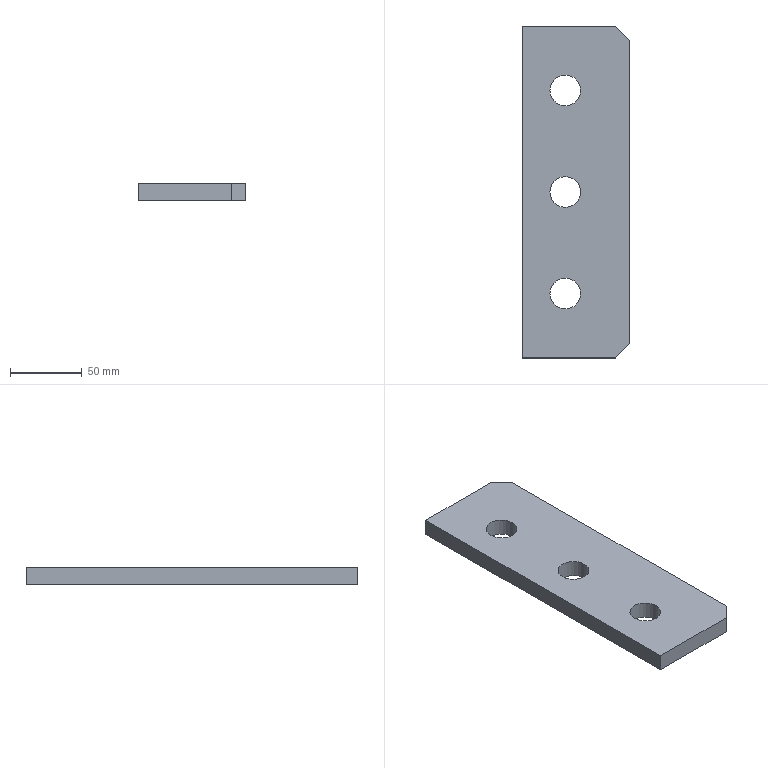Part | STEP file | PN_0021 flange connecting plate 12t_Default<As Machined> | 1 solid | 11 faces | box 75 x 232 x 12 mm | volume 194530 mm3 | plane 8 | cylinder 3 | commonest cylinder face diameters 21.5 x3
STEP:
#1=CARTESIAN_POINT('',(0.,0.,0.));
#2=DIRECTION('',(0.,0.,1.));
#3=DIRECTION('',(1.,0.,0.));
#4=AXIS2_PLACEMENT_3D('',#1,#2,#3);
#5=CARTESIAN_POINT('',(27.5,-116.,0.));
#6=VERTEX_POINT('',#5);
#7=CARTESIAN_POINT('',(27.5,-116.,12.));
#8=VERTEX_POINT('',#7);
#9=CARTESIAN_POINT('',(27.5,-116.,12.));
#10=DIRECTION('',(0.,0.,1.));
#11=VECTOR('',#10,1.);
#12=LINE('',#9,#11);
#13=CARTESIAN_POINT('',(27.5,-116.,12.));
#14=DIRECTION('',(-0.7071,0.7071,0.));
#15=DIRECTION('',(0.,0.,1.));
#16=AXIS2_PLACEMENT_3D('',#13,#14,#15);
#17=PLANE('',#16);
#18=CARTESIAN_POINT('',(0.,0.));
#19=DIRECTION('',(1.,0.));
#20=VECTOR('',#19,1.);
#21=LINE('',#18,#20);
#22=(GEOMETRIC_REPRESENTATION_CONTEXT(2)PARAMETRIC_REPRESENTATION_CONTEXT()REPRESENTATION_CONTEXT('',''));
#23=DEFINITIONAL_REPRESENTATION('',(#21),#22);
#24=PCURVE('',#17,#23);
#25=CARTESIAN_POINT('',(-37.5,-116.,12.));
#26=DIRECTION('',(0.,1.,0.));
#27=DIRECTION('',(0.,0.,1.));
#28=AXIS2_PLACEMENT_3D('',#25,#26,#27);
#29=PLANE('',#28);
#30=CARTESIAN_POINT('',(0.,65.));
#31=DIRECTION('',(1.,0.));
#32=VECTOR('',#31,1.);
#33=LINE('',#30,#32);
#34=(GEOMETRIC_REPRESENTATION_CONTEXT(2)PARAMETRIC_REPRESENTATION_CONTEXT()REPRESENTATION_CONTEXT('',''));
#35=DEFINITIONAL_REPRESENTATION('',(#33),#34);
#36=PCURVE('',#29,#35);
#37=SURFACE_CURVE('',#12,(#24,#36),.PCURVE_S1.);
#38=EDGE_CURVE('',#6,#8,#37,.T.);
#39=ORIENTED_EDGE('',*,*,#38,.F.);
#40=CARTESIAN_POINT('',(37.5,-106.,0.));
#41=VERTEX_POINT('',#40);
#42=CARTESIAN_POINT('',(27.5,-116.,0.));
#43=DIRECTION('',(-0.7071,-0.7071,0.));
#44=VECTOR('',#43,1.);
#45=LINE('',#42,#44);
#46=CARTESIAN_POINT('',(-12.,0.));
#47=DIRECTION('',(0.,-1.));
#48=VECTOR('',#47,1.);
#49=LINE('',#46,#48);
#50=(GEOMETRIC_REPRESENTATION_CONTEXT(2)PARAMETRIC_REPRESENTATION_CONTEXT()REPRESENTATION_CONTEXT('',''));
#51=DEFINITIONAL_REPRESENTATION('',(#49),#50);
#52=PCURVE('',#17,#51);
#53=CARTESIAN_POINT('',(0.,0.,0.));
#54=DIRECTION('',(0.,0.,1.));
#55=DIRECTION('',(1.,0.,0.));
#56=AXIS2_PLACEMENT_3D('',#53,#54,#55);
#57=PLANE('',#56);
#58=CARTESIAN_POINT('',(27.5,-116.));
#59=DIRECTION('',(-0.7071,-0.7071));
#60=VECTOR('',#59,1.);
#61=LINE('',#58,#60);
#62=(GEOMETRIC_REPRESENTATION_CONTEXT(2)PARAMETRIC_REPRESENTATION_CONTEXT()REPRESENTATION_CONTEXT('',''));
#63=DEFINITIONAL_REPRESENTATION('',(#61),#62);
#64=PCURVE('',#57,#63);
#65=SURFACE_CURVE('',#45,(#52,#64),.PCURVE_S1.);
#66=EDGE_CURVE('',#41,#6,#65,.T.);
#67=ORIENTED_EDGE('',*,*,#66,.F.);
#68=CARTESIAN_POINT('',(37.5,-106.,12.));
#69=VERTEX_POINT('',#68);
#70=CARTESIAN_POINT('',(37.5,-106.,12.));
#71=DIRECTION('',(0.,0.,-1.));
#72=VECTOR('',#71,1.);
#73=LINE('',#70,#72);
#74=CARTESIAN_POINT('',(0.,14.142));
#75=DIRECTION('',(-1.,0.));
#76=VECTOR('',#75,1.);
#77=LINE('',#74,#76);
#78=(GEOMETRIC_REPRESENTATION_CONTEXT(2)PARAMETRIC_REPRESENTATION_CONTEXT()REPRESENTATION_CONTEXT('',''));
#79=DEFINITIONAL_REPRESENTATION('',(#77),#78);
#80=PCURVE('',#17,#79);
#81=CARTESIAN_POINT('',(37.5,116.,12.));
#82=DIRECTION('',(-1.,0.,0.));
#83=DIRECTION('',(0.,0.,1.));
#84=AXIS2_PLACEMENT_3D('',#81,#82,#83);
#85=PLANE('',#84);
#86=CARTESIAN_POINT('',(0.,-222.));
#87=DIRECTION('',(-1.,0.));
#88=VECTOR('',#87,1.);
#89=LINE('',#86,#88);
#90=(GEOMETRIC_REPRESENTATION_CONTEXT(2)PARAMETRIC_REPRESENTATION_CONTEXT()REPRESENTATION_CONTEXT('',''));
#91=DEFINITIONAL_REPRESENTATION('',(#89),#90);
#92=PCURVE('',#85,#91);
#93=SURFACE_CURVE('',#73,(#80,#92),.PCURVE_S1.);
#94=EDGE_CURVE('',#69,#41,#93,.T.);
#95=ORIENTED_EDGE('',*,*,#94,.F.);
#96=CARTESIAN_POINT('',(71.75,-71.75,12.));
#97=DIRECTION('',(0.7071,0.7071,0.));
#98=VECTOR('',#97,1.);
#99=LINE('',#96,#98);
#100=CARTESIAN_POINT('',(0.,62.579));
#101=DIRECTION('',(0.,1.));
#102=VECTOR('',#101,1.);
#103=LINE('',#100,#102);
#104=(GEOMETRIC_REPRESENTATION_CONTEXT(2)PARAMETRIC_REPRESENTATION_CONTEXT()REPRESENTATION_CONTEXT('',''));
#105=DEFINITIONAL_REPRESENTATION('',(#103),#104);
#106=PCURVE('',#17,#105);
#107=CARTESIAN_POINT('',(0.,0.,12.));
#108=DIRECTION('',(0.,0.,1.));
#109=DIRECTION('',(1.,0.,0.));
#110=AXIS2_PLACEMENT_3D('',#107,#108,#109);
#111=PLANE('',#110);
#112=CARTESIAN_POINT('',(71.75,-71.75));
#113=DIRECTION('',(0.7071,0.7071));
#114=VECTOR('',#113,1.);
#115=LINE('',#112,#114);
#116=(GEOMETRIC_REPRESENTATION_CONTEXT(2)PARAMETRIC_REPRESENTATION_CONTEXT()REPRESENTATION_CONTEXT('',''));
#117=DEFINITIONAL_REPRESENTATION('',(#115),#116);
#118=PCURVE('',#111,#117);
#119=SURFACE_CURVE('',#99,(#106,#118),.PCURVE_S1.);
#120=EDGE_CURVE('',#8,#69,#119,.T.);
#121=ORIENTED_EDGE('',*,*,#120,.F.);
#122=EDGE_LOOP('',(#39,#67,#95,#121));
#123=FACE_BOUND('',#122,.T.);
#124=ADVANCED_FACE('',(#123),#17,.F.);
#125=CARTESIAN_POINT('',(27.5,116.,12.));
#126=VERTEX_POINT('',#125);
#127=CARTESIAN_POINT('',(27.5,116.,0.));
#128=VERTEX_POINT('',#127);
#129=CARTESIAN_POINT('',(27.5,116.,12.));
#130=DIRECTION('',(0.,0.,-1.));
#131=VECTOR('',#130,1.);
#132=LINE('',#129,#131);
#133=CARTESIAN_POINT('',(27.5,116.,12.));
#134=DIRECTION('',(-0.7071,-0.7071,0.));
#135=DIRECTION('',(0.,0.,-1.));
#136=AXIS2_PLACEMENT_3D('',#133,#134,#135);
#137=PLANE('',#136);
#138=CARTESIAN_POINT('',(0.,0.));
#139=DIRECTION('',(1.,0.));
#140=VECTOR('',#139,1.);
#141=LINE('',#138,#140);
#142=(GEOMETRIC_REPRESENTATION_CONTEXT(2)PARAMETRIC_REPRESENTATION_CONTEXT()REPRESENTATION_CONTEXT('',''));
#143=DEFINITIONAL_REPRESENTATION('',(#141),#142);
#144=PCURVE('',#137,#143);
#145=CARTESIAN_POINT('',(-37.5,116.,12.));
#146=DIRECTION('',(0.,-1.,0.));
#147=DIRECTION('',(0.,0.,-1.));
#148=AXIS2_PLACEMENT_3D('',#145,#146,#147);
#149=PLANE('',#148);
#150=CARTESIAN_POINT('',(0.,65.));
#151=DIRECTION('',(1.,0.));
#152=VECTOR('',#151,1.);
#153=LINE('',#150,#152);
#154=(GEOMETRIC_REPRESENTATION_CONTEXT(2)PARAMETRIC_REPRESENTATION_CONTEXT()REPRESENTATION_CONTEXT('',''));
#155=DEFINITIONAL_REPRESENTATION('',(#153),#154);
#156=PCURVE('',#149,#155);
#157=SURFACE_CURVE('',#132,(#144,#156),.PCURVE_S1.);
#158=EDGE_CURVE('',#126,#128,#157,.T.);
#159=ORIENTED_EDGE('',*,*,#158,.F.);
#160=CARTESIAN_POINT('',(37.5,106.,12.));
#161=VERTEX_POINT('',#160);
#162=CARTESIAN_POINT('',(71.75,71.75,12.));
#163=DIRECTION('',(-0.7071,0.7071,0.));
#164=VECTOR('',#163,1.);
#165=LINE('',#162,#164);
#166=CARTESIAN_POINT('',(0.,62.579));
#167=DIRECTION('',(0.,-1.));
#168=VECTOR('',#167,1.);
#169=LINE('',#166,#168);
#170=(GEOMETRIC_REPRESENTATION_CONTEXT(2)PARAMETRIC_REPRESENTATION_CONTEXT()REPRESENTATION_CONTEXT('',''));
#171=DEFINITIONAL_REPRESENTATION('',(#169),#170);
#172=PCURVE('',#137,#171);
#173=CARTESIAN_POINT('',(71.75,71.75));
#174=DIRECTION('',(-0.7071,0.7071));
#175=VECTOR('',#174,1.);
#176=LINE('',#173,#175);
#177=(GEOMETRIC_REPRESENTATION_CONTEXT(2)PARAMETRIC_REPRESENTATION_CONTEXT()REPRESENTATION_CONTEXT('',''));
#178=DEFINITIONAL_REPRESENTATION('',(#176),#177);
#179=PCURVE('',#111,#178);
#180=SURFACE_CURVE('',#165,(#172,#179),.PCURVE_S1.);
#181=EDGE_CURVE('',#161,#126,#180,.T.);
#182=ORIENTED_EDGE('',*,*,#181,.F.);
#183=CARTESIAN_POINT('',(37.5,106.,0.));
#184=VERTEX_POINT('',#183);
#185=CARTESIAN_POINT('',(37.5,106.,12.));
#186=DIRECTION('',(0.,0.,1.));
#187=VECTOR('',#186,1.);
#188=LINE('',#185,#187);
#189=CARTESIAN_POINT('',(0.,14.142));
#190=DIRECTION('',(-1.,0.));
#191=VECTOR('',#190,1.);
#192=LINE('',#189,#191);
#193=(GEOMETRIC_REPRESENTATION_CONTEXT(2)PARAMETRIC_REPRESENTATION_CONTEXT()REPRESENTATION_CONTEXT('',''));
#194=DEFINITIONAL_REPRESENTATION('',(#192),#193);
#195=PCURVE('',#137,#194);
#196=CARTESIAN_POINT('',(0.,-10.));
#197=DIRECTION('',(1.,0.));
#198=VECTOR('',#197,1.);
#199=LINE('',#196,#198);
#200=(GEOMETRIC_REPRESENTATION_CONTEXT(2)PARAMETRIC_REPRESENTATION_CONTEXT()REPRESENTATION_CONTEXT('',''));
#201=DEFINITIONAL_REPRESENTATION('',(#199),#200);
#202=PCURVE('',#85,#201);
#203=SURFACE_CURVE('',#188,(#195,#202),.PCURVE_S1.);
#204=EDGE_CURVE('',#184,#161,#203,.T.);
#205=ORIENTED_EDGE('',*,*,#204,.F.);
#206=CARTESIAN_POINT('',(27.5,116.,0.));
#207=DIRECTION('',(0.7071,-0.7071,0.));
#208=VECTOR('',#207,1.);
#209=LINE('',#206,#208);
#210=CARTESIAN_POINT('',(12.,0.));
#211=DIRECTION('',(0.,1.));
#212=VECTOR('',#211,1.);
#213=LINE('',#210,#212);
#214=(GEOMETRIC_REPRESENTATION_CONTEXT(2)PARAMETRIC_REPRESENTATION_CONTEXT()REPRESENTATION_CONTEXT('',''));
#215=DEFINITIONAL_REPRESENTATION('',(#213),#214);
#216=PCURVE('',#137,#215);
#217=CARTESIAN_POINT('',(27.5,116.));
#218=DIRECTION('',(0.7071,-0.7071));
#219=VECTOR('',#218,1.);
#220=LINE('',#217,#219);
#221=(GEOMETRIC_REPRESENTATION_CONTEXT(2)PARAMETRIC_REPRESENTATION_CONTEXT()REPRESENTATION_CONTEXT('',''));
#222=DEFINITIONAL_REPRESENTATION('',(#220),#221);
#223=PCURVE('',#57,#222);
#224=SURFACE_CURVE('',#209,(#216,#223),.PCURVE_S1.);
#225=EDGE_CURVE('',#128,#184,#224,.T.);
#226=ORIENTED_EDGE('',*,*,#225,.F.);
#227=EDGE_LOOP('',(#159,#182,#205,#226));
#228=FACE_BOUND('',#227,.T.);
#229=ADVANCED_FACE('',(#228),#137,.F.);
#230=CARTESIAN_POINT('',(37.5,116.,12.));
#231=DIRECTION('',(0.,1.,0.));
#232=VECTOR('',#231,1.);
#233=LINE('',#230,#232);
#234=CARTESIAN_POINT('',(0.,0.));
#235=DIRECTION('',(0.,1.));
#236=VECTOR('',#235,1.);
#237=LINE('',#234,#236);
#238=(GEOMETRIC_REPRESENTATION_CONTEXT(2)PARAMETRIC_REPRESENTATION_CONTEXT()REPRESENTATION_CONTEXT('',''));
#239=DEFINITIONAL_REPRESENTATION('',(#237),#238);
#240=PCURVE('',#85,#239);
#241=CARTESIAN_POINT('',(37.5,116.));
#242=DIRECTION('',(0.,1.));
#243=VECTOR('',#242,1.);
#244=LINE('',#241,#243);
#245=(GEOMETRIC_REPRESENTATION_CONTEXT(2)PARAMETRIC_REPRESENTATION_CONTEXT()REPRESENTATION_CONTEXT('',''));
#246=DEFINITIONAL_REPRESENTATION('',(#244),#245);
#247=PCURVE('',#111,#246);
#248=SURFACE_CURVE('',#233,(#240,#247),.PCURVE_S1.);
#249=EDGE_CURVE('',#69,#161,#248,.T.);
#250=ORIENTED_EDGE('',*,*,#249,.F.);
#251=ORIENTED_EDGE('',*,*,#94,.T.);
#252=CARTESIAN_POINT('',(37.5,116.,0.));
#253=DIRECTION('',(0.,1.,0.));
#254=VECTOR('',#253,1.);
#255=LINE('',#252,#254);
#256=CARTESIAN_POINT('',(-12.,0.));
#257=DIRECTION('',(0.,1.));
#258=VECTOR('',#257,1.);
#259=LINE('',#256,#258);
#260=(GEOMETRIC_REPRESENTATION_CONTEXT(2)PARAMETRIC_REPRESENTATION_CONTEXT()REPRESENTATION_CONTEXT('',''));
#261=DEFINITIONAL_REPRESENTATION('',(#259),#260);
#262=PCURVE('',#85,#261);
#263=CARTESIAN_POINT('',(37.5,116.));
#264=DIRECTION('',(0.,1.));
#265=VECTOR('',#264,1.);
#266=LINE('',#263,#265);
#267=(GEOMETRIC_REPRESENTATION_CONTEXT(2)PARAMETRIC_REPRESENTATION_CONTEXT()REPRESENTATION_CONTEXT('',''));
#268=DEFINITIONAL_REPRESENTATION('',(#266),#267);
#269=PCURVE('',#57,#268);
#270=SURFACE_CURVE('',#255,(#262,#269),.PCURVE_S1.);
#271=EDGE_CURVE('',#41,#184,#270,.T.);
#272=ORIENTED_EDGE('',*,*,#271,.T.);
#273=ORIENTED_EDGE('',*,*,#204,.T.);
#274=EDGE_LOOP('',(#250,#251,#272,#273));
#275=FACE_BOUND('',#274,.T.);
#276=ADVANCED_FACE('',(#275),#85,.F.);
#277=CARTESIAN_POINT('',(-37.5,116.,12.));
#278=VERTEX_POINT('',#277);
#279=CARTESIAN_POINT('',(-37.5,116.,12.));
#280=DIRECTION('',(-1.,0.,0.));
#281=VECTOR('',#280,1.);
#282=LINE('',#279,#281);
#283=CARTESIAN_POINT('',(0.,0.));
#284=DIRECTION('',(0.,-1.));
#285=VECTOR('',#284,1.);
#286=LINE('',#283,#285);
#287=(GEOMETRIC_REPRESENTATION_CONTEXT(2)PARAMETRIC_REPRESENTATION_CONTEXT()REPRESENTATION_CONTEXT('',''));
#288=DEFINITIONAL_REPRESENTATION('',(#286),#287);
#289=PCURVE('',#149,#288);
#290=CARTESIAN_POINT('',(-37.5,116.));
#291=DIRECTION('',(-1.,0.));
#292=VECTOR('',#291,1.);
#293=LINE('',#290,#292);
#294=(GEOMETRIC_REPRESENTATION_CONTEXT(2)PARAMETRIC_REPRESENTATION_CONTEXT()REPRESENTATION_CONTEXT('',''));
#295=DEFINITIONAL_REPRESENTATION('',(#293),#294);
#296=PCURVE('',#111,#295);
#297=SURFACE_CURVE('',#282,(#289,#296),.PCURVE_S1.);
#298=EDGE_CURVE('',#126,#278,#297,.T.);
#299=ORIENTED_EDGE('',*,*,#298,.F.);
#300=ORIENTED_EDGE('',*,*,#158,.T.);
#301=CARTESIAN_POINT('',(-37.5,116.,0.));
#302=VERTEX_POINT('',#301);
#303=CARTESIAN_POINT('',(-37.5,116.,0.));
#304=DIRECTION('',(-1.,0.,0.));
#305=VECTOR('',#304,1.);
#306=LINE('',#303,#305);
#307=CARTESIAN_POINT('',(12.,0.));
#308=DIRECTION('',(0.,-1.));
#309=VECTOR('',#308,1.);
#310=LINE('',#307,#309);
#311=(GEOMETRIC_REPRESENTATION_CONTEXT(2)PARAMETRIC_REPRESENTATION_CONTEXT()REPRESENTATION_CONTEXT('',''));
#312=DEFINITIONAL_REPRESENTATION('',(#310),#311);
#313=PCURVE('',#149,#312);
#314=CARTESIAN_POINT('',(-37.5,116.));
#315=DIRECTION('',(-1.,0.));
#316=VECTOR('',#315,1.);
#317=LINE('',#314,#316);
#318=(GEOMETRIC_REPRESENTATION_CONTEXT(2)PARAMETRIC_REPRESENTATION_CONTEXT()REPRESENTATION_CONTEXT('',''));
#319=DEFINITIONAL_REPRESENTATION('',(#317),#318);
#320=PCURVE('',#57,#319);
#321=SURFACE_CURVE('',#306,(#313,#320),.PCURVE_S1.);
#322=EDGE_CURVE('',#128,#302,#321,.T.);
#323=ORIENTED_EDGE('',*,*,#322,.T.);
#324=CARTESIAN_POINT('',(-37.5,116.,12.));
#325=DIRECTION('',(0.,0.,-1.));
#326=VECTOR('',#325,1.);
#327=LINE('',#324,#326);
#328=CARTESIAN_POINT('',(0.,0.));
#329=DIRECTION('',(1.,0.));
#330=VECTOR('',#329,1.);
#331=LINE('',#328,#330);
#332=(GEOMETRIC_REPRESENTATION_CONTEXT(2)PARAMETRIC_REPRESENTATION_CONTEXT()REPRESENTATION_CONTEXT('',''));
#333=DEFINITIONAL_REPRESENTATION('',(#331),#332);
#334=PCURVE('',#149,#333);
#335=CARTESIAN_POINT('',(-37.5,116.,12.));
#336=DIRECTION('',(1.,0.,0.));
#337=DIRECTION('',(0.,0.,-1.));
#338=AXIS2_PLACEMENT_3D('',#335,#336,#337);
#339=PLANE('',#338);
#340=CARTESIAN_POINT('',(0.,0.));
#341=DIRECTION('',(1.,0.));
#342=VECTOR('',#341,1.);
#343=LINE('',#340,#342);
#344=(GEOMETRIC_REPRESENTATION_CONTEXT(2)PARAMETRIC_REPRESENTATION_CONTEXT()REPRESENTATION_CONTEXT('',''));
#345=DEFINITIONAL_REPRESENTATION('',(#343),#344);
#346=PCURVE('',#339,#345);
#347=SURFACE_CURVE('',#327,(#334,#346),.PCURVE_S1.);
#348=EDGE_CURVE('',#278,#302,#347,.T.);
#349=ORIENTED_EDGE('',*,*,#348,.F.);
#350=EDGE_LOOP('',(#299,#300,#323,#349));
#351=FACE_BOUND('',#350,.T.);
#352=ADVANCED_FACE('',(#351),#149,.F.);
#353=CARTESIAN_POINT('',(-37.5,-116.,0.));
#354=VERTEX_POINT('',#353);
#355=CARTESIAN_POINT('',(-37.5,116.,0.));
#356=DIRECTION('',(0.,-1.,0.));
#357=VECTOR('',#356,1.);
#358=LINE('',#355,#357);
#359=CARTESIAN_POINT('',(12.,0.));
#360=DIRECTION('',(0.,-1.));
#361=VECTOR('',#360,1.);
#362=LINE('',#359,#361);
#363=(GEOMETRIC_REPRESENTATION_CONTEXT(2)PARAMETRIC_REPRESENTATION_CONTEXT()REPRESENTATION_CONTEXT('',''));
#364=DEFINITIONAL_REPRESENTATION('',(#362),#363);
#365=PCURVE('',#339,#364);
#366=CARTESIAN_POINT('',(-37.5,116.));
#367=DIRECTION('',(0.,-1.));
#368=VECTOR('',#367,1.);
#369=LINE('',#366,#368);
#370=(GEOMETRIC_REPRESENTATION_CONTEXT(2)PARAMETRIC_REPRESENTATION_CONTEXT()REPRESENTATION_CONTEXT('',''));
#371=DEFINITIONAL_REPRESENTATION('',(#369),#370);
#372=PCURVE('',#57,#371);
#373=SURFACE_CURVE('',#358,(#365,#372),.PCURVE_S1.);
#374=EDGE_CURVE('',#302,#354,#373,.T.);
#375=ORIENTED_EDGE('',*,*,#374,.T.);
#376=CARTESIAN_POINT('',(-37.5,-116.,12.));
#377=VERTEX_POINT('',#376);
#378=CARTESIAN_POINT('',(-37.5,-116.,12.));
#379=DIRECTION('',(0.,0.,-1.));
#380=VECTOR('',#379,1.);
#381=LINE('',#378,#380);
#382=CARTESIAN_POINT('',(0.,-232.));
#383=DIRECTION('',(1.,0.));
#384=VECTOR('',#383,1.);
#385=LINE('',#382,#384);
#386=(GEOMETRIC_REPRESENTATION_CONTEXT(2)PARAMETRIC_REPRESENTATION_CONTEXT()REPRESENTATION_CONTEXT('',''));
#387=DEFINITIONAL_REPRESENTATION('',(#385),#386);
#388=PCURVE('',#339,#387);
#389=CARTESIAN_POINT('',(0.,0.));
#390=DIRECTION('',(-1.,0.));
#391=VECTOR('',#390,1.);
#392=LINE('',#389,#391);
#393=(GEOMETRIC_REPRESENTATION_CONTEXT(2)PARAMETRIC_REPRESENTATION_CONTEXT()REPRESENTATION_CONTEXT('',''));
#394=DEFINITIONAL_REPRESENTATION('',(#392),#393);
#395=PCURVE('',#29,#394);
#396=SURFACE_CURVE('',#381,(#388,#395),.PCURVE_S1.);
#397=EDGE_CURVE('',#377,#354,#396,.T.);
#398=ORIENTED_EDGE('',*,*,#397,.F.);
#399=CARTESIAN_POINT('',(-37.5,116.,12.));
#400=DIRECTION('',(0.,-1.,0.));
#401=VECTOR('',#400,1.);
#402=LINE('',#399,#401);
#403=CARTESIAN_POINT('',(0.,0.));
#404=DIRECTION('',(0.,-1.));
#405=VECTOR('',#404,1.);
#406=LINE('',#403,#405);
#407=(GEOMETRIC_REPRESENTATION_CONTEXT(2)PARAMETRIC_REPRESENTATION_CONTEXT()REPRESENTATION_CONTEXT('',''));
#408=DEFINITIONAL_REPRESENTATION('',(#406),#407);
#409=PCURVE('',#339,#408);
#410=CARTESIAN_POINT('',(-37.5,116.));
#411=DIRECTION('',(0.,-1.));
#412=VECTOR('',#411,1.);
#413=LINE('',#410,#412);
#414=(GEOMETRIC_REPRESENTATION_CONTEXT(2)PARAMETRIC_REPRESENTATION_CONTEXT()REPRESENTATION_CONTEXT('',''));
#415=DEFINITIONAL_REPRESENTATION('',(#413),#414);
#416=PCURVE('',#111,#415);
#417=SURFACE_CURVE('',#402,(#409,#416),.PCURVE_S1.);
#418=EDGE_CURVE('',#278,#377,#417,.T.);
#419=ORIENTED_EDGE('',*,*,#418,.F.);
#420=ORIENTED_EDGE('',*,*,#348,.T.);
#421=EDGE_LOOP('',(#375,#398,#419,#420));
#422=FACE_BOUND('',#421,.T.);
#423=ADVANCED_FACE('',(#422),#339,.F.);
#424=CARTESIAN_POINT('',(-37.5,-116.,0.));
#425=DIRECTION('',(1.,0.,0.));
#426=VECTOR('',#425,1.);
#427=LINE('',#424,#426);
#428=CARTESIAN_POINT('',(-12.,0.));
#429=DIRECTION('',(0.,1.));
#430=VECTOR('',#429,1.);
#431=LINE('',#428,#430);
#432=(GEOMETRIC_REPRESENTATION_CONTEXT(2)PARAMETRIC_REPRESENTATION_CONTEXT()REPRESENTATION_CONTEXT('',''));
#433=DEFINITIONAL_REPRESENTATION('',(#431),#432);
#434=PCURVE('',#29,#433);
#435=CARTESIAN_POINT('',(-37.5,-116.));
#436=DIRECTION('',(1.,0.));
#437=VECTOR('',#436,1.);
#438=LINE('',#435,#437);
#439=(GEOMETRIC_REPRESENTATION_CONTEXT(2)PARAMETRIC_REPRESENTATION_CONTEXT()REPRESENTATION_CONTEXT('',''));
#440=DEFINITIONAL_REPRESENTATION('',(#438),#439);
#441=PCURVE('',#57,#440);
#442=SURFACE_CURVE('',#427,(#434,#441),.PCURVE_S1.);
#443=EDGE_CURVE('',#354,#6,#442,.T.);
#444=ORIENTED_EDGE('',*,*,#443,.T.);
#445=ORIENTED_EDGE('',*,*,#38,.T.);
#446=CARTESIAN_POINT('',(-37.5,-116.,12.));
#447=DIRECTION('',(1.,0.,0.));
#448=VECTOR('',#447,1.);
#449=LINE('',#446,#448);
#450=CARTESIAN_POINT('',(0.,0.));
#451=DIRECTION('',(0.,1.));
#452=VECTOR('',#451,1.);
#453=LINE('',#450,#452);
#454=(GEOMETRIC_REPRESENTATION_CONTEXT(2)PARAMETRIC_REPRESENTATION_CONTEXT()REPRESENTATION_CONTEXT('',''));
#455=DEFINITIONAL_REPRESENTATION('',(#453),#454);
#456=PCURVE('',#29,#455);
#457=CARTESIAN_POINT('',(-37.5,-116.));
#458=DIRECTION('',(1.,0.));
#459=VECTOR('',#458,1.);
#460=LINE('',#457,#459);
#461=(GEOMETRIC_REPRESENTATION_CONTEXT(2)PARAMETRIC_REPRESENTATION_CONTEXT()REPRESENTATION_CONTEXT('',''));
#462=DEFINITIONAL_REPRESENTATION('',(#460),#461);
#463=PCURVE('',#111,#462);
#464=SURFACE_CURVE('',#449,(#456,#463),.PCURVE_S1.);
#465=EDGE_CURVE('',#377,#8,#464,.T.);
#466=ORIENTED_EDGE('',*,*,#465,.F.);
#467=ORIENTED_EDGE('',*,*,#397,.T.);
#468=EDGE_LOOP('',(#444,#445,#466,#467));
#469=FACE_BOUND('',#468,.T.);
#470=ADVANCED_FACE('',(#469),#29,.F.);
#471=CARTESIAN_POINT('',(3.25,71.,12.));
#472=VERTEX_POINT('',#471);
#473=CARTESIAN_POINT('',(-7.5,71.,12.));
#474=DIRECTION('',(0.,0.,1.));
#475=DIRECTION('',(1.,0.,0.));
#476=AXIS2_PLACEMENT_3D('',#473,#474,#475);
#477=CIRCLE('',#476,10.75);
#478=CARTESIAN_POINT('',(-7.5,71.));
#479=DIRECTION('',(1.,0.));
#480=AXIS2_PLACEMENT_2D('',#478,#479);
#481=CIRCLE('',#480,10.75);
#482=(GEOMETRIC_REPRESENTATION_CONTEXT(2)PARAMETRIC_REPRESENTATION_CONTEXT()REPRESENTATION_CONTEXT('',''));
#483=DEFINITIONAL_REPRESENTATION('',(#481),#482);
#484=PCURVE('',#111,#483);
#485=CARTESIAN_POINT('',(-7.5,71.,12.));
#486=DIRECTION('',(0.,0.,1.));
#487=DIRECTION('',(1.,0.,0.));
#488=AXIS2_PLACEMENT_3D('',#485,#486,#487);
#489=CYLINDRICAL_SURFACE('',#488,10.75);
#490=CARTESIAN_POINT('',(0.,0.));
#491=DIRECTION('',(1.,0.));
#492=VECTOR('',#491,1.);
#493=LINE('',#490,#492);
#494=(GEOMETRIC_REPRESENTATION_CONTEXT(2)PARAMETRIC_REPRESENTATION_CONTEXT()REPRESENTATION_CONTEXT('',''));
#495=DEFINITIONAL_REPRESENTATION('',(#493),#494);
#496=PCURVE('',#489,#495);
#497=SURFACE_CURVE('',#477,(#484,#496),.PCURVE_S1.);
#498=EDGE_CURVE('',#472,#472,#497,.T.);
#499=ORIENTED_EDGE('',*,*,#498,.F.);
#500=EDGE_LOOP('',(#499));
#501=FACE_BOUND('',#500,.T.);
#502=CARTESIAN_POINT('',(3.25,0.,12.));
#503=VERTEX_POINT('',#502);
#504=CARTESIAN_POINT('',(-7.5,0.,12.));
#505=DIRECTION('',(0.,0.,1.));
#506=DIRECTION('',(1.,0.,0.));
#507=AXIS2_PLACEMENT_3D('',#504,#505,#506);
#508=CIRCLE('',#507,10.75);
#509=CARTESIAN_POINT('',(-7.5,0.));
#510=DIRECTION('',(1.,0.));
#511=AXIS2_PLACEMENT_2D('',#509,#510);
#512=CIRCLE('',#511,10.75);
#513=(GEOMETRIC_REPRESENTATION_CONTEXT(2)PARAMETRIC_REPRESENTATION_CONTEXT()REPRESENTATION_CONTEXT('',''));
#514=DEFINITIONAL_REPRESENTATION('',(#512),#513);
#515=PCURVE('',#111,#514);
#516=CARTESIAN_POINT('',(-7.5,0.,12.));
#517=DIRECTION('',(0.,0.,1.));
#518=DIRECTION('',(1.,0.,0.));
#519=AXIS2_PLACEMENT_3D('',#516,#517,#518);
#520=CYLINDRICAL_SURFACE('',#519,10.75);
#521=CARTESIAN_POINT('',(0.,0.));
#522=DIRECTION('',(1.,0.));
#523=VECTOR('',#522,1.);
#524=LINE('',#521,#523);
#525=(GEOMETRIC_REPRESENTATION_CONTEXT(2)PARAMETRIC_REPRESENTATION_CONTEXT()REPRESENTATION_CONTEXT('',''));
#526=DEFINITIONAL_REPRESENTATION('',(#524),#525);
#527=PCURVE('',#520,#526);
#528=SURFACE_CURVE('',#508,(#515,#527),.PCURVE_S1.);
#529=EDGE_CURVE('',#503,#503,#528,.T.);
#530=ORIENTED_EDGE('',*,*,#529,.F.);
#531=EDGE_LOOP('',(#530));
#532=FACE_BOUND('',#531,.T.);
#533=CARTESIAN_POINT('',(3.25,-71.,12.));
#534=VERTEX_POINT('',#533);
#535=CARTESIAN_POINT('',(-7.5,-71.,12.));
#536=DIRECTION('',(0.,0.,1.));
#537=DIRECTION('',(1.,0.,0.));
#538=AXIS2_PLACEMENT_3D('',#535,#536,#537);
#539=CIRCLE('',#538,10.75);
#540=CARTESIAN_POINT('',(-7.5,-71.));
#541=DIRECTION('',(1.,0.));
#542=AXIS2_PLACEMENT_2D('',#540,#541);
#543=CIRCLE('',#542,10.75);
#544=(GEOMETRIC_REPRESENTATION_CONTEXT(2)PARAMETRIC_REPRESENTATION_CONTEXT()REPRESENTATION_CONTEXT('',''));
#545=DEFINITIONAL_REPRESENTATION('',(#543),#544);
#546=PCURVE('',#111,#545);
#547=CARTESIAN_POINT('',(-7.5,-71.,12.));
#548=DIRECTION('',(0.,0.,1.));
#549=DIRECTION('',(1.,0.,0.));
#550=AXIS2_PLACEMENT_3D('',#547,#548,#549);
#551=CYLINDRICAL_SURFACE('',#550,10.75);
#552=CARTESIAN_POINT('',(0.,0.));
#553=DIRECTION('',(1.,0.));
#554=VECTOR('',#553,1.);
#555=LINE('',#552,#554);
#556=(GEOMETRIC_REPRESENTATION_CONTEXT(2)PARAMETRIC_REPRESENTATION_CONTEXT()REPRESENTATION_CONTEXT('',''));
#557=DEFINITIONAL_REPRESENTATION('',(#555),#556);
#558=PCURVE('',#551,#557);
#559=SURFACE_CURVE('',#539,(#546,#558),.PCURVE_S1.);
#560=EDGE_CURVE('',#534,#534,#559,.T.);
#561=ORIENTED_EDGE('',*,*,#560,.F.);
#562=EDGE_LOOP('',(#561));
#563=FACE_BOUND('',#562,.T.);
#564=ORIENTED_EDGE('',*,*,#465,.T.);
#565=ORIENTED_EDGE('',*,*,#120,.T.);
#566=ORIENTED_EDGE('',*,*,#249,.T.);
#567=ORIENTED_EDGE('',*,*,#181,.T.);
#568=ORIENTED_EDGE('',*,*,#298,.T.);
#569=ORIENTED_EDGE('',*,*,#418,.T.);
#570=EDGE_LOOP('',(#564,#565,#566,#567,#568,#569));
#571=FACE_BOUND('',#570,.T.);
#572=ADVANCED_FACE('',(#501,#532,#563,#571),#111,.T.);
#573=CARTESIAN_POINT('',(3.25,71.,0.));
#574=VERTEX_POINT('',#573);
#575=CARTESIAN_POINT('',(-7.5,71.,0.));
#576=DIRECTION('',(0.,0.,1.));
#577=DIRECTION('',(1.,0.,0.));
#578=AXIS2_PLACEMENT_3D('',#575,#576,#577);
#579=CIRCLE('',#578,10.75);
#580=CARTESIAN_POINT('',(-7.5,71.));
#581=DIRECTION('',(1.,0.));
#582=AXIS2_PLACEMENT_2D('',#580,#581);
#583=CIRCLE('',#582,10.75);
#584=(GEOMETRIC_REPRESENTATION_CONTEXT(2)PARAMETRIC_REPRESENTATION_CONTEXT()REPRESENTATION_CONTEXT('',''));
#585=DEFINITIONAL_REPRESENTATION('',(#583),#584);
#586=PCURVE('',#57,#585);
#587=CARTESIAN_POINT('',(0.,-12.));
#588=DIRECTION('',(1.,0.));
#589=VECTOR('',#588,1.);
#590=LINE('',#587,#589);
#591=(GEOMETRIC_REPRESENTATION_CONTEXT(2)PARAMETRIC_REPRESENTATION_CONTEXT()REPRESENTATION_CONTEXT('',''));
#592=DEFINITIONAL_REPRESENTATION('',(#590),#591);
#593=PCURVE('',#489,#592);
#594=SURFACE_CURVE('',#579,(#586,#593),.PCURVE_S1.);
#595=EDGE_CURVE('',#574,#574,#594,.T.);
#596=ORIENTED_EDGE('',*,*,#595,.T.);
#597=EDGE_LOOP('',(#596));
#598=FACE_BOUND('',#597,.T.);
#599=CARTESIAN_POINT('',(3.25,0.,0.));
#600=VERTEX_POINT('',#599);
#601=CARTESIAN_POINT('',(-7.5,0.,0.));
#602=DIRECTION('',(0.,0.,1.));
#603=DIRECTION('',(1.,0.,0.));
#604=AXIS2_PLACEMENT_3D('',#601,#602,#603);
#605=CIRCLE('',#604,10.75);
#606=CARTESIAN_POINT('',(-7.5,0.));
#607=DIRECTION('',(1.,0.));
#608=AXIS2_PLACEMENT_2D('',#606,#607);
#609=CIRCLE('',#608,10.75);
#610=(GEOMETRIC_REPRESENTATION_CONTEXT(2)PARAMETRIC_REPRESENTATION_CONTEXT()REPRESENTATION_CONTEXT('',''));
#611=DEFINITIONAL_REPRESENTATION('',(#609),#610);
#612=PCURVE('',#57,#611);
#613=CARTESIAN_POINT('',(0.,-12.));
#614=DIRECTION('',(1.,0.));
#615=VECTOR('',#614,1.);
#616=LINE('',#613,#615);
#617=(GEOMETRIC_REPRESENTATION_CONTEXT(2)PARAMETRIC_REPRESENTATION_CONTEXT()REPRESENTATION_CONTEXT('',''));
#618=DEFINITIONAL_REPRESENTATION('',(#616),#617);
#619=PCURVE('',#520,#618);
#620=SURFACE_CURVE('',#605,(#612,#619),.PCURVE_S1.);
#621=EDGE_CURVE('',#600,#600,#620,.T.);
#622=ORIENTED_EDGE('',*,*,#621,.T.);
#623=EDGE_LOOP('',(#622));
#624=FACE_BOUND('',#623,.T.);
#625=CARTESIAN_POINT('',(3.25,-71.,0.));
#626=VERTEX_POINT('',#625);
#627=CARTESIAN_POINT('',(-7.5,-71.,0.));
#628=DIRECTION('',(0.,0.,1.));
#629=DIRECTION('',(1.,0.,0.));
#630=AXIS2_PLACEMENT_3D('',#627,#628,#629);
#631=CIRCLE('',#630,10.75);
#632=CARTESIAN_POINT('',(-7.5,-71.));
#633=DIRECTION('',(1.,0.));
#634=AXIS2_PLACEMENT_2D('',#632,#633);
#635=CIRCLE('',#634,10.75);
#636=(GEOMETRIC_REPRESENTATION_CONTEXT(2)PARAMETRIC_REPRESENTATION_CONTEXT()REPRESENTATION_CONTEXT('',''));
#637=DEFINITIONAL_REPRESENTATION('',(#635),#636);
#638=PCURVE('',#57,#637);
#639=CARTESIAN_POINT('',(0.,-12.));
#640=DIRECTION('',(1.,0.));
#641=VECTOR('',#640,1.);
#642=LINE('',#639,#641);
#643=(GEOMETRIC_REPRESENTATION_CONTEXT(2)PARAMETRIC_REPRESENTATION_CONTEXT()REPRESENTATION_CONTEXT('',''));
#644=DEFINITIONAL_REPRESENTATION('',(#642),#643);
#645=PCURVE('',#551,#644);
#646=SURFACE_CURVE('',#631,(#638,#645),.PCURVE_S1.);
#647=EDGE_CURVE('',#626,#626,#646,.T.);
#648=ORIENTED_EDGE('',*,*,#647,.T.);
#649=EDGE_LOOP('',(#648));
#650=FACE_BOUND('',#649,.T.);
#651=ORIENTED_EDGE('',*,*,#271,.F.);
#652=ORIENTED_EDGE('',*,*,#66,.T.);
#653=ORIENTED_EDGE('',*,*,#443,.F.);
#654=ORIENTED_EDGE('',*,*,#374,.F.);
#655=ORIENTED_EDGE('',*,*,#322,.F.);
#656=ORIENTED_EDGE('',*,*,#225,.T.);
#657=EDGE_LOOP('',(#651,#652,#653,#654,#655,#656));
#658=FACE_BOUND('',#657,.T.);
#659=ADVANCED_FACE('',(#598,#624,#650,#658),#57,.F.);
#660=ORIENTED_EDGE('',*,*,#560,.F.);
#661=CARTESIAN_POINT('',(3.25,-71.,0.));
#662=CARTESIAN_POINT('',(3.25,-71.,12.));
#663=B_SPLINE_CURVE_WITH_KNOTS('',1,(#661,#662),.UNSPECIFIED.,.F.,.F.,(2,2),(-12.,0.),.PIECEWISE_BEZIER_KNOTS.);
#664=CARTESIAN_POINT('',(0.,0.));
#665=DIRECTION('',(0.,1.));
#666=VECTOR('',#665,1.);
#667=LINE('',#664,#666);
#668=(GEOMETRIC_REPRESENTATION_CONTEXT(2)PARAMETRIC_REPRESENTATION_CONTEXT()REPRESENTATION_CONTEXT('',''));
#669=DEFINITIONAL_REPRESENTATION('',(#667),#668);
#670=PCURVE('',#551,#669);
#671=CARTESIAN_POINT('',(6.283,0.));
#672=DIRECTION('',(0.,1.));
#673=VECTOR('',#672,1.);
#674=LINE('',#671,#673);
#675=(GEOMETRIC_REPRESENTATION_CONTEXT(2)PARAMETRIC_REPRESENTATION_CONTEXT()REPRESENTATION_CONTEXT('',''));
#676=DEFINITIONAL_REPRESENTATION('',(#674),#675);
#677=PCURVE('',#551,#676);
#678=SEAM_CURVE('',#663,(#670,#677),.PCURVE_S1.);
#679=EDGE_CURVE('',#626,#534,#678,.T.);
#680=ORIENTED_EDGE('',*,*,#679,.F.);
#681=ORIENTED_EDGE('',*,*,#647,.T.);
#682=ORIENTED_EDGE('',*,*,#679,.T.);
#683=EDGE_LOOP('',(#660,#680,#681,#682));
#684=FACE_BOUND('',#683,.F.);
#685=ADVANCED_FACE('',(#684),#551,.F.);
#686=ORIENTED_EDGE('',*,*,#529,.F.);
#687=CARTESIAN_POINT('',(3.25,0.,0.));
#688=CARTESIAN_POINT('',(3.25,0.,12.));
#689=B_SPLINE_CURVE_WITH_KNOTS('',1,(#687,#688),.UNSPECIFIED.,.F.,.F.,(2,2),(-12.,0.),.PIECEWISE_BEZIER_KNOTS.);
#690=CARTESIAN_POINT('',(0.,0.));
#691=DIRECTION('',(0.,1.));
#692=VECTOR('',#691,1.);
#693=LINE('',#690,#692);
#694=(GEOMETRIC_REPRESENTATION_CONTEXT(2)PARAMETRIC_REPRESENTATION_CONTEXT()REPRESENTATION_CONTEXT('',''));
#695=DEFINITIONAL_REPRESENTATION('',(#693),#694);
#696=PCURVE('',#520,#695);
#697=CARTESIAN_POINT('',(6.283,0.));
#698=DIRECTION('',(0.,1.));
#699=VECTOR('',#698,1.);
#700=LINE('',#697,#699);
#701=(GEOMETRIC_REPRESENTATION_CONTEXT(2)PARAMETRIC_REPRESENTATION_CONTEXT()REPRESENTATION_CONTEXT('',''));
#702=DEFINITIONAL_REPRESENTATION('',(#700),#701);
#703=PCURVE('',#520,#702);
#704=SEAM_CURVE('',#689,(#696,#703),.PCURVE_S1.);
#705=EDGE_CURVE('',#600,#503,#704,.T.);
#706=ORIENTED_EDGE('',*,*,#705,.F.);
#707=ORIENTED_EDGE('',*,*,#621,.T.);
#708=ORIENTED_EDGE('',*,*,#705,.T.);
#709=EDGE_LOOP('',(#686,#706,#707,#708));
#710=FACE_BOUND('',#709,.F.);
#711=ADVANCED_FACE('',(#710),#520,.F.);
#712=ORIENTED_EDGE('',*,*,#498,.F.);
#713=CARTESIAN_POINT('',(3.25,71.,0.));
#714=CARTESIAN_POINT('',(3.25,71.,12.));
#715=B_SPLINE_CURVE_WITH_KNOTS('',1,(#713,#714),.UNSPECIFIED.,.F.,.F.,(2,2),(-12.,0.),.PIECEWISE_BEZIER_KNOTS.);
#716=CARTESIAN_POINT('',(0.,0.));
#717=DIRECTION('',(0.,1.));
#718=VECTOR('',#717,1.);
#719=LINE('',#716,#718);
#720=(GEOMETRIC_REPRESENTATION_CONTEXT(2)PARAMETRIC_REPRESENTATION_CONTEXT()REPRESENTATION_CONTEXT('',''));
#721=DEFINITIONAL_REPRESENTATION('',(#719),#720);
#722=PCURVE('',#489,#721);
#723=CARTESIAN_POINT('',(6.283,0.));
#724=DIRECTION('',(0.,1.));
#725=VECTOR('',#724,1.);
#726=LINE('',#723,#725);
#727=(GEOMETRIC_REPRESENTATION_CONTEXT(2)PARAMETRIC_REPRESENTATION_CONTEXT()REPRESENTATION_CONTEXT('',''));
#728=DEFINITIONAL_REPRESENTATION('',(#726),#727);
#729=PCURVE('',#489,#728);
#730=SEAM_CURVE('',#715,(#722,#729),.PCURVE_S1.);
#731=EDGE_CURVE('',#574,#472,#730,.T.);
#732=ORIENTED_EDGE('',*,*,#731,.F.);
#733=ORIENTED_EDGE('',*,*,#595,.T.);
#734=ORIENTED_EDGE('',*,*,#731,.T.);
#735=EDGE_LOOP('',(#712,#732,#733,#734));
#736=FACE_BOUND('',#735,.F.);
#737=ADVANCED_FACE('',(#736),#489,.F.);
#738=CLOSED_SHELL('',(#124,#229,#276,#352,#423,#470,#572,#659,#685,#711,#737));
#739=MANIFOLD_SOLID_BREP('',#738);
#740=(LENGTH_UNIT()NAMED_UNIT(*)SI_UNIT(.MILLI.,.METRE.));
#741=UNCERTAINTY_MEASURE_WITH_UNIT(LENGTH_MEASURE(0.000002),#740,'','');
#742=(NAMED_UNIT(*)PLANE_ANGLE_UNIT()SI_UNIT($,.RADIAN.));
#743=(NAMED_UNIT(*)SI_UNIT($,.STERADIAN.)SOLID_ANGLE_UNIT());
#744=(GEOMETRIC_REPRESENTATION_CONTEXT(3)GLOBAL_UNCERTAINTY_ASSIGNED_CONTEXT((#741))GLOBAL_UNIT_ASSIGNED_CONTEXT((#740,#742,#743))REPRESENTATION_CONTEXT('',''));
#745=ADVANCED_BREP_SHAPE_REPRESENTATION('',(#4,#739),#744);